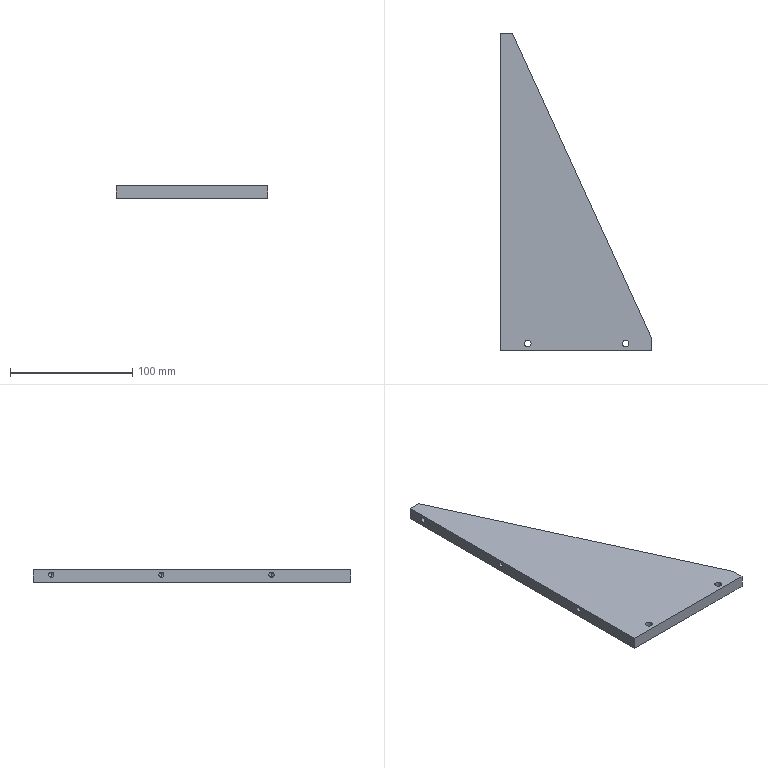Part | STEP file | FBDS-JIN | 1 solid | 29 faces | box 124 x 260 x 10 mm | volume 178303 mm3 | cylinder 14 | plane 9 | cone 6 | commonest cylinder face diameters 4.2 x6 5.5 x4 9.8 x4
STEP:
#1=CARTESIAN_POINT('',(107.4,6.,5.7));
#2=VERTEX_POINT('',#1);
#3=CARTESIAN_POINT('',(97.6,6.,5.7));
#4=VERTEX_POINT('',#3);
#5=CARTESIAN_POINT('',(102.5,6.,5.7));
#6=DIRECTION('',(0.,0.,-1.));
#7=DIRECTION('',(-1.,0.,0.));
#8=AXIS2_PLACEMENT_3D('',#5,#6,#7);
#9=CIRCLE('',#8,4.9);
#10=EDGE_CURVE('',#2,#4,#9,.T.);
#11=ORIENTED_EDGE('',*,*,#10,.F.);
#12=CARTESIAN_POINT('',(107.4,6.,0.));
#13=VERTEX_POINT('',#12);
#14=CARTESIAN_POINT('',(107.4,6.,0.));
#15=DIRECTION('',(0.,0.,-1.));
#16=VECTOR('',#15,1000.);
#17=LINE('',#14,#16);
#18=EDGE_CURVE('',#2,#13,#17,.T.);
#19=ORIENTED_EDGE('',*,*,#18,.T.);
#20=CARTESIAN_POINT('',(97.6,6.,0.));
#21=VERTEX_POINT('',#20);
#22=CARTESIAN_POINT('',(102.5,6.,0.));
#23=DIRECTION('',(0.,0.,-1.));
#24=DIRECTION('',(-1.,0.,0.));
#25=AXIS2_PLACEMENT_3D('',#22,#23,#24);
#26=CIRCLE('',#25,4.9);
#27=EDGE_CURVE('',#13,#21,#26,.T.);
#28=ORIENTED_EDGE('',*,*,#27,.T.);
#29=CARTESIAN_POINT('',(97.6,6.,0.));
#30=DIRECTION('',(0.,0.,-1.));
#31=VECTOR('',#30,1000.);
#32=LINE('',#29,#31);
#33=EDGE_CURVE('',#4,#21,#32,.T.);
#34=ORIENTED_EDGE('',*,*,#33,.F.);
#35=EDGE_LOOP('',(#11,#19,#28,#34));
#36=FACE_OUTER_BOUND('',#35,.T.);
#37=CARTESIAN_POINT('',(102.5,6.,0.));
#38=DIRECTION('',(0.,0.,-1.));
#39=DIRECTION('',(-1.,0.,0.));
#40=AXIS2_PLACEMENT_3D('',#37,#38,#39);
#41=CYLINDRICAL_SURFACE('',#40,4.9);
#42=ADVANCED_FACE('',(#36),#41,.F.);
#43=CARTESIAN_POINT('',(105.25,6.,10.));
#44=VERTEX_POINT('',#43);
#45=CARTESIAN_POINT('',(99.75,6.,10.));
#46=VERTEX_POINT('',#45);
#47=CARTESIAN_POINT('',(102.5,6.,10.));
#48=DIRECTION('',(0.,0.,-1.));
#49=DIRECTION('',(-1.,0.,0.));
#50=AXIS2_PLACEMENT_3D('',#47,#48,#49);
#51=CIRCLE('',#50,2.75);
#52=EDGE_CURVE('',#44,#46,#51,.T.);
#53=ORIENTED_EDGE('',*,*,#52,.F.);
#54=CARTESIAN_POINT('',(105.25,6.,5.7));
#55=VERTEX_POINT('',#54);
#56=CARTESIAN_POINT('',(105.25,6.,0.));
#57=DIRECTION('',(0.,0.,-1.));
#58=VECTOR('',#57,1000.);
#59=LINE('',#56,#58);
#60=EDGE_CURVE('',#44,#55,#59,.T.);
#61=ORIENTED_EDGE('',*,*,#60,.T.);
#62=CARTESIAN_POINT('',(99.75,6.,5.7));
#63=VERTEX_POINT('',#62);
#64=CARTESIAN_POINT('',(102.5,6.,5.7));
#65=DIRECTION('',(0.,0.,-1.));
#66=DIRECTION('',(-1.,0.,0.));
#67=AXIS2_PLACEMENT_3D('',#64,#65,#66);
#68=CIRCLE('',#67,2.75);
#69=EDGE_CURVE('',#55,#63,#68,.T.);
#70=ORIENTED_EDGE('',*,*,#69,.T.);
#71=CARTESIAN_POINT('',(99.75,6.,0.));
#72=DIRECTION('',(0.,0.,-1.));
#73=VECTOR('',#72,1000.);
#74=LINE('',#71,#73);
#75=EDGE_CURVE('',#46,#63,#74,.T.);
#76=ORIENTED_EDGE('',*,*,#75,.F.);
#77=EDGE_LOOP('',(#53,#61,#70,#76));
#78=FACE_OUTER_BOUND('',#77,.T.);
#79=CARTESIAN_POINT('',(102.5,6.,0.));
#80=DIRECTION('',(0.,0.,-1.));
#81=DIRECTION('',(-1.,0.,0.));
#82=AXIS2_PLACEMENT_3D('',#79,#80,#81);
#83=CYLINDRICAL_SURFACE('',#82,2.75);
#84=ADVANCED_FACE('',(#78),#83,.F.);
#85=CARTESIAN_POINT('',(27.4,6.,5.7));
#86=VERTEX_POINT('',#85);
#87=CARTESIAN_POINT('',(17.6,6.,5.7));
#88=VERTEX_POINT('',#87);
#89=CARTESIAN_POINT('',(22.5,6.,5.7));
#90=DIRECTION('',(0.,0.,-1.));
#91=DIRECTION('',(-1.,0.,0.));
#92=AXIS2_PLACEMENT_3D('',#89,#90,#91);
#93=CIRCLE('',#92,4.9);
#94=EDGE_CURVE('',#86,#88,#93,.T.);
#95=ORIENTED_EDGE('',*,*,#94,.F.);
#96=CARTESIAN_POINT('',(27.4,6.,0.));
#97=VERTEX_POINT('',#96);
#98=CARTESIAN_POINT('',(27.4,6.,0.));
#99=DIRECTION('',(0.,0.,-1.));
#100=VECTOR('',#99,1000.);
#101=LINE('',#98,#100);
#102=EDGE_CURVE('',#86,#97,#101,.T.);
#103=ORIENTED_EDGE('',*,*,#102,.T.);
#104=CARTESIAN_POINT('',(17.6,6.,0.));
#105=VERTEX_POINT('',#104);
#106=CARTESIAN_POINT('',(22.5,6.,0.));
#107=DIRECTION('',(0.,0.,-1.));
#108=DIRECTION('',(-1.,0.,0.));
#109=AXIS2_PLACEMENT_3D('',#106,#107,#108);
#110=CIRCLE('',#109,4.9);
#111=EDGE_CURVE('',#97,#105,#110,.T.);
#112=ORIENTED_EDGE('',*,*,#111,.T.);
#113=CARTESIAN_POINT('',(17.6,6.,0.));
#114=DIRECTION('',(0.,0.,-1.));
#115=VECTOR('',#114,1000.);
#116=LINE('',#113,#115);
#117=EDGE_CURVE('',#88,#105,#116,.T.);
#118=ORIENTED_EDGE('',*,*,#117,.F.);
#119=EDGE_LOOP('',(#95,#103,#112,#118));
#120=FACE_OUTER_BOUND('',#119,.T.);
#121=CARTESIAN_POINT('',(22.5,6.,0.));
#122=DIRECTION('',(0.,0.,-1.));
#123=DIRECTION('',(-1.,0.,0.));
#124=AXIS2_PLACEMENT_3D('',#121,#122,#123);
#125=CYLINDRICAL_SURFACE('',#124,4.9);
#126=ADVANCED_FACE('',(#120),#125,.F.);
#127=CARTESIAN_POINT('',(25.25,6.,10.));
#128=VERTEX_POINT('',#127);
#129=CARTESIAN_POINT('',(19.75,6.,10.));
#130=VERTEX_POINT('',#129);
#131=CARTESIAN_POINT('',(22.5,6.,10.));
#132=DIRECTION('',(0.,0.,-1.));
#133=DIRECTION('',(-1.,0.,0.));
#134=AXIS2_PLACEMENT_3D('',#131,#132,#133);
#135=CIRCLE('',#134,2.75);
#136=EDGE_CURVE('',#128,#130,#135,.T.);
#137=ORIENTED_EDGE('',*,*,#136,.F.);
#138=CARTESIAN_POINT('',(25.25,6.,5.7));
#139=VERTEX_POINT('',#138);
#140=CARTESIAN_POINT('',(25.25,6.,0.));
#141=DIRECTION('',(0.,0.,-1.));
#142=VECTOR('',#141,1000.);
#143=LINE('',#140,#142);
#144=EDGE_CURVE('',#128,#139,#143,.T.);
#145=ORIENTED_EDGE('',*,*,#144,.T.);
#146=CARTESIAN_POINT('',(19.75,6.,5.7));
#147=VERTEX_POINT('',#146);
#148=CARTESIAN_POINT('',(22.5,6.,5.7));
#149=DIRECTION('',(0.,0.,-1.));
#150=DIRECTION('',(-1.,0.,0.));
#151=AXIS2_PLACEMENT_3D('',#148,#149,#150);
#152=CIRCLE('',#151,2.75);
#153=EDGE_CURVE('',#139,#147,#152,.T.);
#154=ORIENTED_EDGE('',*,*,#153,.T.);
#155=CARTESIAN_POINT('',(19.75,6.,0.));
#156=DIRECTION('',(0.,0.,-1.));
#157=VECTOR('',#156,1000.);
#158=LINE('',#155,#157);
#159=EDGE_CURVE('',#130,#147,#158,.T.);
#160=ORIENTED_EDGE('',*,*,#159,.F.);
#161=EDGE_LOOP('',(#137,#145,#154,#160));
#162=FACE_OUTER_BOUND('',#161,.T.);
#163=CARTESIAN_POINT('',(22.5,6.,0.));
#164=DIRECTION('',(0.,0.,-1.));
#165=DIRECTION('',(-1.,0.,0.));
#166=AXIS2_PLACEMENT_3D('',#163,#164,#165);
#167=CYLINDRICAL_SURFACE('',#166,2.75);
#168=ADVANCED_FACE('',(#162),#167,.F.);
#169=CARTESIAN_POINT('',(12.4,245.,3.9));
#170=VERTEX_POINT('',#169);
#171=CARTESIAN_POINT('',(12.4,245.,8.1));
#172=VERTEX_POINT('',#171);
#173=CARTESIAN_POINT('',(12.4,245.,6.));
#174=DIRECTION('',(-1.,0.,0.));
#175=DIRECTION('',(0.,0.,1.));
#176=AXIS2_PLACEMENT_3D('',#173,#174,#175);
#177=CIRCLE('',#176,2.1);
#178=EDGE_CURVE('',#170,#172,#177,.T.);
#179=ORIENTED_EDGE('',*,*,#178,.F.);
#180=CARTESIAN_POINT('',(0.,245.,3.9));
#181=VERTEX_POINT('',#180);
#182=CARTESIAN_POINT('',(0.,245.,3.9));
#183=DIRECTION('',(-1.,0.,0.));
#184=VECTOR('',#183,1000.);
#185=LINE('',#182,#184);
#186=EDGE_CURVE('',#170,#181,#185,.T.);
#187=ORIENTED_EDGE('',*,*,#186,.T.);
#188=CARTESIAN_POINT('',(0.,245.,8.1));
#189=VERTEX_POINT('',#188);
#190=CARTESIAN_POINT('',(0.,245.,6.));
#191=DIRECTION('',(-1.,0.,0.));
#192=DIRECTION('',(0.,0.,1.));
#193=AXIS2_PLACEMENT_3D('',#190,#191,#192);
#194=CIRCLE('',#193,2.1);
#195=EDGE_CURVE('',#181,#189,#194,.T.);
#196=ORIENTED_EDGE('',*,*,#195,.T.);
#197=CARTESIAN_POINT('',(0.,245.,8.1));
#198=DIRECTION('',(-1.,0.,0.));
#199=VECTOR('',#198,1000.);
#200=LINE('',#197,#199);
#201=EDGE_CURVE('',#172,#189,#200,.T.);
#202=ORIENTED_EDGE('',*,*,#201,.F.);
#203=EDGE_LOOP('',(#179,#187,#196,#202));
#204=FACE_OUTER_BOUND('',#203,.T.);
#205=CARTESIAN_POINT('',(0.,245.,6.));
#206=DIRECTION('',(-1.,0.,0.));
#207=DIRECTION('',(0.,0.,1.));
#208=AXIS2_PLACEMENT_3D('',#205,#206,#207);
#209=CYLINDRICAL_SURFACE('',#208,2.1);
#210=ADVANCED_FACE('',(#204),#209,.F.);
#211=CARTESIAN_POINT('',(13.662,245.,6.));
#212=VERTEX_POINT('',#211);
#213=CARTESIAN_POINT('',(12.4,245.,8.1));
#214=DIRECTION('',(-0.515,0.,0.8572));
#215=VECTOR('',#214,1000.);
#216=LINE('',#213,#215);
#217=EDGE_CURVE('',#212,#172,#216,.T.);
#218=ORIENTED_EDGE('',*,*,#217,.F.);
#219=CARTESIAN_POINT('',(12.4,245.,3.9));
#220=DIRECTION('',(-0.515,0.,-0.8572));
#221=VECTOR('',#220,1000.);
#222=LINE('',#219,#221);
#223=EDGE_CURVE('',#212,#170,#222,.T.);
#224=ORIENTED_EDGE('',*,*,#223,.T.);
#225=ORIENTED_EDGE('',*,*,#178,.T.);
#226=EDGE_LOOP('',(#218,#224,#225));
#227=FACE_OUTER_BOUND('',#226,.T.);
#228=CARTESIAN_POINT('',(12.4,245.,6.));
#229=DIRECTION('',(-1.,0.,0.));
#230=DIRECTION('',(0.,0.,1.));
#231=AXIS2_PLACEMENT_3D('',#228,#229,#230);
#232=CONICAL_SURFACE('',#231,2.1,1.03);
#233=ADVANCED_FACE('',(#227),#232,.F.);
#234=CARTESIAN_POINT('',(12.4,155.,3.9));
#235=VERTEX_POINT('',#234);
#236=CARTESIAN_POINT('',(12.4,155.,8.1));
#237=VERTEX_POINT('',#236);
#238=CARTESIAN_POINT('',(12.4,155.,6.));
#239=DIRECTION('',(-1.,0.,0.));
#240=DIRECTION('',(0.,0.,1.));
#241=AXIS2_PLACEMENT_3D('',#238,#239,#240);
#242=CIRCLE('',#241,2.1);
#243=EDGE_CURVE('',#235,#237,#242,.T.);
#244=ORIENTED_EDGE('',*,*,#243,.F.);
#245=CARTESIAN_POINT('',(0.,155.,3.9));
#246=VERTEX_POINT('',#245);
#247=CARTESIAN_POINT('',(0.,155.,3.9));
#248=DIRECTION('',(-1.,0.,0.));
#249=VECTOR('',#248,1000.);
#250=LINE('',#247,#249);
#251=EDGE_CURVE('',#235,#246,#250,.T.);
#252=ORIENTED_EDGE('',*,*,#251,.T.);
#253=CARTESIAN_POINT('',(0.,155.,8.1));
#254=VERTEX_POINT('',#253);
#255=CARTESIAN_POINT('',(0.,155.,6.));
#256=DIRECTION('',(-1.,0.,0.));
#257=DIRECTION('',(0.,0.,1.));
#258=AXIS2_PLACEMENT_3D('',#255,#256,#257);
#259=CIRCLE('',#258,2.1);
#260=EDGE_CURVE('',#246,#254,#259,.T.);
#261=ORIENTED_EDGE('',*,*,#260,.T.);
#262=CARTESIAN_POINT('',(0.,155.,8.1));
#263=DIRECTION('',(-1.,0.,0.));
#264=VECTOR('',#263,1000.);
#265=LINE('',#262,#264);
#266=EDGE_CURVE('',#237,#254,#265,.T.);
#267=ORIENTED_EDGE('',*,*,#266,.F.);
#268=EDGE_LOOP('',(#244,#252,#261,#267));
#269=FACE_OUTER_BOUND('',#268,.T.);
#270=CARTESIAN_POINT('',(0.,155.,6.));
#271=DIRECTION('',(-1.,0.,0.));
#272=DIRECTION('',(0.,0.,1.));
#273=AXIS2_PLACEMENT_3D('',#270,#271,#272);
#274=CYLINDRICAL_SURFACE('',#273,2.1);
#275=ADVANCED_FACE('',(#269),#274,.F.);
#276=CARTESIAN_POINT('',(13.662,155.,6.));
#277=VERTEX_POINT('',#276);
#278=CARTESIAN_POINT('',(12.4,155.,8.1));
#279=DIRECTION('',(-0.515,0.,0.8572));
#280=VECTOR('',#279,1000.);
#281=LINE('',#278,#280);
#282=EDGE_CURVE('',#277,#237,#281,.T.);
#283=ORIENTED_EDGE('',*,*,#282,.F.);
#284=CARTESIAN_POINT('',(12.4,155.,3.9));
#285=DIRECTION('',(-0.515,0.,-0.8572));
#286=VECTOR('',#285,1000.);
#287=LINE('',#284,#286);
#288=EDGE_CURVE('',#277,#235,#287,.T.);
#289=ORIENTED_EDGE('',*,*,#288,.T.);
#290=ORIENTED_EDGE('',*,*,#243,.T.);
#291=EDGE_LOOP('',(#283,#289,#290));
#292=FACE_OUTER_BOUND('',#291,.T.);
#293=CARTESIAN_POINT('',(12.4,155.,6.));
#294=DIRECTION('',(-1.,0.,0.));
#295=DIRECTION('',(0.,0.,1.));
#296=AXIS2_PLACEMENT_3D('',#293,#294,#295);
#297=CONICAL_SURFACE('',#296,2.1,1.03);
#298=ADVANCED_FACE('',(#292),#297,.F.);
#299=CARTESIAN_POINT('',(12.4,65.,3.9));
#300=VERTEX_POINT('',#299);
#301=CARTESIAN_POINT('',(12.4,65.,8.1));
#302=VERTEX_POINT('',#301);
#303=CARTESIAN_POINT('',(12.4,65.,6.));
#304=DIRECTION('',(-1.,0.,0.));
#305=DIRECTION('',(0.,0.,1.));
#306=AXIS2_PLACEMENT_3D('',#303,#304,#305);
#307=CIRCLE('',#306,2.1);
#308=EDGE_CURVE('',#300,#302,#307,.T.);
#309=ORIENTED_EDGE('',*,*,#308,.F.);
#310=CARTESIAN_POINT('',(0.,65.,3.9));
#311=VERTEX_POINT('',#310);
#312=CARTESIAN_POINT('',(0.,65.,3.9));
#313=DIRECTION('',(-1.,0.,0.));
#314=VECTOR('',#313,1000.);
#315=LINE('',#312,#314);
#316=EDGE_CURVE('',#300,#311,#315,.T.);
#317=ORIENTED_EDGE('',*,*,#316,.T.);
#318=CARTESIAN_POINT('',(0.,65.,8.1));
#319=VERTEX_POINT('',#318);
#320=CARTESIAN_POINT('',(0.,65.,6.));
#321=DIRECTION('',(-1.,0.,0.));
#322=DIRECTION('',(0.,0.,1.));
#323=AXIS2_PLACEMENT_3D('',#320,#321,#322);
#324=CIRCLE('',#323,2.1);
#325=EDGE_CURVE('',#311,#319,#324,.T.);
#326=ORIENTED_EDGE('',*,*,#325,.T.);
#327=CARTESIAN_POINT('',(0.,65.,8.1));
#328=DIRECTION('',(-1.,0.,0.));
#329=VECTOR('',#328,1000.);
#330=LINE('',#327,#329);
#331=EDGE_CURVE('',#302,#319,#330,.T.);
#332=ORIENTED_EDGE('',*,*,#331,.F.);
#333=EDGE_LOOP('',(#309,#317,#326,#332));
#334=FACE_OUTER_BOUND('',#333,.T.);
#335=CARTESIAN_POINT('',(0.,65.,6.));
#336=DIRECTION('',(-1.,0.,0.));
#337=DIRECTION('',(0.,0.,1.));
#338=AXIS2_PLACEMENT_3D('',#335,#336,#337);
#339=CYLINDRICAL_SURFACE('',#338,2.1);
#340=ADVANCED_FACE('',(#334),#339,.F.);
#341=CARTESIAN_POINT('',(13.662,65.,6.));
#342=VERTEX_POINT('',#341);
#343=CARTESIAN_POINT('',(12.4,65.,8.1));
#344=DIRECTION('',(-0.515,0.,0.8572));
#345=VECTOR('',#344,1000.);
#346=LINE('',#343,#345);
#347=EDGE_CURVE('',#342,#302,#346,.T.);
#348=ORIENTED_EDGE('',*,*,#347,.F.);
#349=CARTESIAN_POINT('',(12.4,65.,3.9));
#350=DIRECTION('',(-0.515,0.,-0.8572));
#351=VECTOR('',#350,1000.);
#352=LINE('',#349,#351);
#353=EDGE_CURVE('',#342,#300,#352,.T.);
#354=ORIENTED_EDGE('',*,*,#353,.T.);
#355=ORIENTED_EDGE('',*,*,#308,.T.);
#356=EDGE_LOOP('',(#348,#354,#355));
#357=FACE_OUTER_BOUND('',#356,.T.);
#358=CARTESIAN_POINT('',(12.4,65.,6.));
#359=DIRECTION('',(-1.,0.,0.));
#360=DIRECTION('',(0.,0.,1.));
#361=AXIS2_PLACEMENT_3D('',#358,#359,#360);
#362=CONICAL_SURFACE('',#361,2.1,1.03);
#363=ADVANCED_FACE('',(#357),#362,.F.);
#364=CARTESIAN_POINT('',(0.,245.,6.));
#365=DIRECTION('',(-1.,0.,0.));
#366=DIRECTION('',(0.,0.,1.));
#367=AXIS2_PLACEMENT_3D('',#364,#365,#366);
#368=CIRCLE('',#367,2.1);
#369=EDGE_CURVE('',#189,#181,#368,.T.);
#370=ORIENTED_EDGE('',*,*,#369,.F.);
#371=ORIENTED_EDGE('',*,*,#195,.F.);
#372=EDGE_LOOP('',(#370,#371));
#373=FACE_BOUND('',#372,.T.);
#374=CARTESIAN_POINT('',(0.,155.,6.));
#375=DIRECTION('',(-1.,0.,0.));
#376=DIRECTION('',(0.,0.,1.));
#377=AXIS2_PLACEMENT_3D('',#374,#375,#376);
#378=CIRCLE('',#377,2.1);
#379=EDGE_CURVE('',#254,#246,#378,.T.);
#380=ORIENTED_EDGE('',*,*,#379,.F.);
#381=ORIENTED_EDGE('',*,*,#260,.F.);
#382=EDGE_LOOP('',(#380,#381));
#383=FACE_BOUND('',#382,.T.);
#384=CARTESIAN_POINT('',(0.,65.,6.));
#385=DIRECTION('',(-1.,0.,0.));
#386=DIRECTION('',(0.,0.,1.));
#387=AXIS2_PLACEMENT_3D('',#384,#385,#386);
#388=CIRCLE('',#387,2.1);
#389=EDGE_CURVE('',#319,#311,#388,.T.);
#390=ORIENTED_EDGE('',*,*,#389,.F.);
#391=ORIENTED_EDGE('',*,*,#325,.F.);
#392=EDGE_LOOP('',(#390,#391));
#393=FACE_BOUND('',#392,.T.);
#394=CARTESIAN_POINT('',(0.,260.,0.));
#395=VERTEX_POINT('',#394);
#396=CARTESIAN_POINT('',(0.,0.,0.));
#397=VERTEX_POINT('',#396);
#398=CARTESIAN_POINT('',(0.,0.,0.));
#399=DIRECTION('',(0.,-1.,0.));
#400=VECTOR('',#399,1000.);
#401=LINE('',#398,#400);
#402=EDGE_CURVE('',#395,#397,#401,.T.);
#403=ORIENTED_EDGE('',*,*,#402,.T.);
#404=CARTESIAN_POINT('',(0.,0.,10.));
#405=VERTEX_POINT('',#404);
#406=CARTESIAN_POINT('',(0.,0.,10.));
#407=DIRECTION('',(0.,0.,-1.));
#408=VECTOR('',#407,1000.);
#409=LINE('',#406,#408);
#410=EDGE_CURVE('',#405,#397,#409,.T.);
#411=ORIENTED_EDGE('',*,*,#410,.F.);
#412=CARTESIAN_POINT('',(0.,260.,10.));
#413=VERTEX_POINT('',#412);
#414=CARTESIAN_POINT('',(0.,0.,10.));
#415=DIRECTION('',(0.,-1.,0.));
#416=VECTOR('',#415,1000.);
#417=LINE('',#414,#416);
#418=EDGE_CURVE('',#413,#405,#417,.T.);
#419=ORIENTED_EDGE('',*,*,#418,.F.);
#420=CARTESIAN_POINT('',(0.,260.,10.));
#421=DIRECTION('',(0.,0.,-1.));
#422=VECTOR('',#421,1000.);
#423=LINE('',#420,#422);
#424=EDGE_CURVE('',#413,#395,#423,.T.);
#425=ORIENTED_EDGE('',*,*,#424,.T.);
#426=EDGE_LOOP('',(#403,#411,#419,#425));
#427=FACE_OUTER_BOUND('',#426,.T.);
#428=CARTESIAN_POINT('',(0.,0.,10.));
#429=DIRECTION('',(1.,0.,0.));
#430=DIRECTION('',(0.,0.,-1.));
#431=AXIS2_PLACEMENT_3D('',#428,#429,#430);
#432=PLANE('',#431);
#433=ADVANCED_FACE('',(#373,#383,#393,#427),#432,.F.);
#434=CARTESIAN_POINT('',(124.,0.,0.));
#435=VERTEX_POINT('',#434);
#436=CARTESIAN_POINT('',(0.,0.,0.));
#437=DIRECTION('',(1.,0.,0.));
#438=VECTOR('',#437,1000.);
#439=LINE('',#436,#438);
#440=EDGE_CURVE('',#397,#435,#439,.T.);
#441=ORIENTED_EDGE('',*,*,#440,.T.);
#442=CARTESIAN_POINT('',(124.,0.,10.));
#443=VERTEX_POINT('',#442);
#444=CARTESIAN_POINT('',(124.,0.,10.));
#445=DIRECTION('',(0.,0.,-1.));
#446=VECTOR('',#445,1000.);
#447=LINE('',#444,#446);
#448=EDGE_CURVE('',#443,#435,#447,.T.);
#449=ORIENTED_EDGE('',*,*,#448,.F.);
#450=CARTESIAN_POINT('',(0.,0.,10.));
#451=DIRECTION('',(1.,0.,0.));
#452=VECTOR('',#451,1000.);
#453=LINE('',#450,#452);
#454=EDGE_CURVE('',#405,#443,#453,.T.);
#455=ORIENTED_EDGE('',*,*,#454,.F.);
#456=ORIENTED_EDGE('',*,*,#410,.T.);
#457=EDGE_LOOP('',(#441,#449,#455,#456));
#458=FACE_OUTER_BOUND('',#457,.T.);
#459=CARTESIAN_POINT('',(0.,0.,10.));
#460=DIRECTION('',(0.,1.,0.));
#461=DIRECTION('',(0.,0.,1.));
#462=AXIS2_PLACEMENT_3D('',#459,#460,#461);
#463=PLANE('',#462);
#464=ADVANCED_FACE('',(#458),#463,.F.);
#465=CARTESIAN_POINT('',(124.,10.,0.));
#466=VERTEX_POINT('',#465);
#467=CARTESIAN_POINT('',(124.,0.,0.));
#468=DIRECTION('',(0.,1.,0.));
#469=VECTOR('',#468,1000.);
#470=LINE('',#467,#469);
#471=EDGE_CURVE('',#435,#466,#470,.T.);
#472=ORIENTED_EDGE('',*,*,#471,.T.);
#473=CARTESIAN_POINT('',(124.,10.,10.));
#474=VERTEX_POINT('',#473);
#475=CARTESIAN_POINT('',(124.,10.,10.));
#476=DIRECTION('',(0.,0.,-1.));
#477=VECTOR('',#476,1000.);
#478=LINE('',#475,#477);
#479=EDGE_CURVE('',#474,#466,#478,.T.);
#480=ORIENTED_EDGE('',*,*,#479,.F.);
#481=CARTESIAN_POINT('',(124.,0.,10.));
#482=DIRECTION('',(0.,1.,0.));
#483=VECTOR('',#482,1000.);
#484=LINE('',#481,#483);
#485=EDGE_CURVE('',#443,#474,#484,.T.);
#486=ORIENTED_EDGE('',*,*,#485,.F.);
#487=ORIENTED_EDGE('',*,*,#448,.T.);
#488=EDGE_LOOP('',(#472,#480,#486,#487));
#489=FACE_OUTER_BOUND('',#488,.T.);
#490=CARTESIAN_POINT('',(124.,0.,10.));
#491=DIRECTION('',(-1.,0.,0.));
#492=DIRECTION('',(0.,0.,1.));
#493=AXIS2_PLACEMENT_3D('',#490,#491,#492);
#494=PLANE('',#493);
#495=ADVANCED_FACE('',(#489),#494,.F.);
#496=CARTESIAN_POINT('',(10.,260.,0.));
#497=VERTEX_POINT('',#496);
#498=CARTESIAN_POINT('',(124.,10.,0.));
#499=DIRECTION('',(-0.4149,0.9099,0.));
#500=VECTOR('',#499,1000.);
#501=LINE('',#498,#500);
#502=EDGE_CURVE('',#466,#497,#501,.T.);
#503=ORIENTED_EDGE('',*,*,#502,.T.);
#504=CARTESIAN_POINT('',(10.,260.,10.));
#505=VERTEX_POINT('',#504);
#506=CARTESIAN_POINT('',(10.,260.,10.));
#507=DIRECTION('',(0.,0.,-1.));
#508=VECTOR('',#507,1000.);
#509=LINE('',#506,#508);
#510=EDGE_CURVE('',#505,#497,#509,.T.);
#511=ORIENTED_EDGE('',*,*,#510,.F.);
#512=CARTESIAN_POINT('',(124.,10.,10.));
#513=DIRECTION('',(-0.4149,0.9099,0.));
#514=VECTOR('',#513,1000.);
#515=LINE('',#512,#514);
#516=EDGE_CURVE('',#474,#505,#515,.T.);
#517=ORIENTED_EDGE('',*,*,#516,.F.);
#518=ORIENTED_EDGE('',*,*,#479,.T.);
#519=EDGE_LOOP('',(#503,#511,#517,#518));
#520=FACE_OUTER_BOUND('',#519,.T.);
#521=CARTESIAN_POINT('',(124.,10.,10.));
#522=DIRECTION('',(-0.9099,-0.4149,0.));
#523=DIRECTION('',(0.4149,-0.9099,0.));
#524=AXIS2_PLACEMENT_3D('',#521,#522,#523);
#525=PLANE('',#524);
#526=ADVANCED_FACE('',(#520),#525,.F.);
#527=CARTESIAN_POINT('',(0.,260.,0.));
#528=DIRECTION('',(-1.,0.,0.));
#529=VECTOR('',#528,1000.);
#530=LINE('',#527,#529);
#531=EDGE_CURVE('',#497,#395,#530,.T.);
#532=ORIENTED_EDGE('',*,*,#531,.T.);
#533=ORIENTED_EDGE('',*,*,#424,.F.);
#534=CARTESIAN_POINT('',(0.,260.,10.));
#535=DIRECTION('',(-1.,0.,0.));
#536=VECTOR('',#535,1000.);
#537=LINE('',#534,#536);
#538=EDGE_CURVE('',#505,#413,#537,.T.);
#539=ORIENTED_EDGE('',*,*,#538,.F.);
#540=ORIENTED_EDGE('',*,*,#510,.T.);
#541=EDGE_LOOP('',(#532,#533,#539,#540));
#542=FACE_OUTER_BOUND('',#541,.T.);
#543=CARTESIAN_POINT('',(0.,260.,10.));
#544=DIRECTION('',(0.,-1.,0.));
#545=DIRECTION('',(0.,0.,-1.));
#546=AXIS2_PLACEMENT_3D('',#543,#544,#545);
#547=PLANE('',#546);
#548=ADVANCED_FACE('',(#542),#547,.F.);
#549=CARTESIAN_POINT('',(102.5,6.,10.));
#550=DIRECTION('',(0.,0.,-1.));
#551=DIRECTION('',(-1.,0.,0.));
#552=AXIS2_PLACEMENT_3D('',#549,#550,#551);
#553=CIRCLE('',#552,2.75);
#554=EDGE_CURVE('',#46,#44,#553,.T.);
#555=ORIENTED_EDGE('',*,*,#554,.T.);
#556=ORIENTED_EDGE('',*,*,#52,.T.);
#557=EDGE_LOOP('',(#555,#556));
#558=FACE_BOUND('',#557,.T.);
#559=CARTESIAN_POINT('',(22.5,6.,10.));
#560=DIRECTION('',(0.,0.,-1.));
#561=DIRECTION('',(-1.,0.,0.));
#562=AXIS2_PLACEMENT_3D('',#559,#560,#561);
#563=CIRCLE('',#562,2.75);
#564=EDGE_CURVE('',#130,#128,#563,.T.);
#565=ORIENTED_EDGE('',*,*,#564,.T.);
#566=ORIENTED_EDGE('',*,*,#136,.T.);
#567=EDGE_LOOP('',(#565,#566));
#568=FACE_BOUND('',#567,.T.);
#569=ORIENTED_EDGE('',*,*,#418,.T.);
#570=ORIENTED_EDGE('',*,*,#454,.T.);
#571=ORIENTED_EDGE('',*,*,#485,.T.);
#572=ORIENTED_EDGE('',*,*,#516,.T.);
#573=ORIENTED_EDGE('',*,*,#538,.T.);
#574=EDGE_LOOP('',(#569,#570,#571,#572,#573));
#575=FACE_OUTER_BOUND('',#574,.T.);
#576=CARTESIAN_POINT('',(0.,0.,10.));
#577=DIRECTION('',(0.,0.,-1.));
#578=DIRECTION('',(-1.,0.,0.));
#579=AXIS2_PLACEMENT_3D('',#576,#577,#578);
#580=PLANE('',#579);
#581=ADVANCED_FACE('',(#558,#568,#575),#580,.F.);
#582=CARTESIAN_POINT('',(102.5,6.,0.));
#583=DIRECTION('',(0.,0.,-1.));
#584=DIRECTION('',(-1.,0.,0.));
#585=AXIS2_PLACEMENT_3D('',#582,#583,#584);
#586=CIRCLE('',#585,4.9);
#587=EDGE_CURVE('',#21,#13,#586,.T.);
#588=ORIENTED_EDGE('',*,*,#587,.F.);
#589=ORIENTED_EDGE('',*,*,#27,.F.);
#590=EDGE_LOOP('',(#588,#589));
#591=FACE_BOUND('',#590,.T.);
#592=CARTESIAN_POINT('',(22.5,6.,0.));
#593=DIRECTION('',(0.,0.,-1.));
#594=DIRECTION('',(-1.,0.,0.));
#595=AXIS2_PLACEMENT_3D('',#592,#593,#594);
#596=CIRCLE('',#595,4.9);
#597=EDGE_CURVE('',#105,#97,#596,.T.);
#598=ORIENTED_EDGE('',*,*,#597,.F.);
#599=ORIENTED_EDGE('',*,*,#111,.F.);
#600=EDGE_LOOP('',(#598,#599));
#601=FACE_BOUND('',#600,.T.);
#602=ORIENTED_EDGE('',*,*,#402,.F.);
#603=ORIENTED_EDGE('',*,*,#531,.F.);
#604=ORIENTED_EDGE('',*,*,#502,.F.);
#605=ORIENTED_EDGE('',*,*,#471,.F.);
#606=ORIENTED_EDGE('',*,*,#440,.F.);
#607=EDGE_LOOP('',(#602,#603,#604,#605,#606));
#608=FACE_OUTER_BOUND('',#607,.T.);
#609=CARTESIAN_POINT('',(0.,0.,0.));
#610=DIRECTION('',(0.,0.,-1.));
#611=DIRECTION('',(-1.,0.,0.));
#612=AXIS2_PLACEMENT_3D('',#609,#610,#611);
#613=PLANE('',#612);
#614=ADVANCED_FACE('',(#591,#601,#608),#613,.T.);
#615=ORIENTED_EDGE('',*,*,#353,.F.);
#616=ORIENTED_EDGE('',*,*,#347,.T.);
#617=CARTESIAN_POINT('',(12.4,65.,6.));
#618=DIRECTION('',(-1.,0.,0.));
#619=DIRECTION('',(0.,0.,1.));
#620=AXIS2_PLACEMENT_3D('',#617,#618,#619);
#621=CIRCLE('',#620,2.1);
#622=EDGE_CURVE('',#302,#300,#621,.T.);
#623=ORIENTED_EDGE('',*,*,#622,.T.);
#624=EDGE_LOOP('',(#615,#616,#623));
#625=FACE_OUTER_BOUND('',#624,.T.);
#626=CARTESIAN_POINT('',(12.4,65.,6.));
#627=DIRECTION('',(-1.,0.,0.));
#628=DIRECTION('',(0.,0.,1.));
#629=AXIS2_PLACEMENT_3D('',#626,#627,#628);
#630=CONICAL_SURFACE('',#629,2.1,1.03);
#631=ADVANCED_FACE('',(#625),#630,.F.);
#632=ORIENTED_EDGE('',*,*,#316,.F.);
#633=ORIENTED_EDGE('',*,*,#622,.F.);
#634=ORIENTED_EDGE('',*,*,#331,.T.);
#635=ORIENTED_EDGE('',*,*,#389,.T.);
#636=EDGE_LOOP('',(#632,#633,#634,#635));
#637=FACE_OUTER_BOUND('',#636,.T.);
#638=CARTESIAN_POINT('',(0.,65.,6.));
#639=DIRECTION('',(-1.,0.,0.));
#640=DIRECTION('',(0.,0.,1.));
#641=AXIS2_PLACEMENT_3D('',#638,#639,#640);
#642=CYLINDRICAL_SURFACE('',#641,2.1);
#643=ADVANCED_FACE('',(#637),#642,.F.);
#644=ORIENTED_EDGE('',*,*,#288,.F.);
#645=ORIENTED_EDGE('',*,*,#282,.T.);
#646=CARTESIAN_POINT('',(12.4,155.,6.));
#647=DIRECTION('',(-1.,0.,0.));
#648=DIRECTION('',(0.,0.,1.));
#649=AXIS2_PLACEMENT_3D('',#646,#647,#648);
#650=CIRCLE('',#649,2.1);
#651=EDGE_CURVE('',#237,#235,#650,.T.);
#652=ORIENTED_EDGE('',*,*,#651,.T.);
#653=EDGE_LOOP('',(#644,#645,#652));
#654=FACE_OUTER_BOUND('',#653,.T.);
#655=CARTESIAN_POINT('',(12.4,155.,6.));
#656=DIRECTION('',(-1.,0.,0.));
#657=DIRECTION('',(0.,0.,1.));
#658=AXIS2_PLACEMENT_3D('',#655,#656,#657);
#659=CONICAL_SURFACE('',#658,2.1,1.03);
#660=ADVANCED_FACE('',(#654),#659,.F.);
#661=ORIENTED_EDGE('',*,*,#251,.F.);
#662=ORIENTED_EDGE('',*,*,#651,.F.);
#663=ORIENTED_EDGE('',*,*,#266,.T.);
#664=ORIENTED_EDGE('',*,*,#379,.T.);
#665=EDGE_LOOP('',(#661,#662,#663,#664));
#666=FACE_OUTER_BOUND('',#665,.T.);
#667=CARTESIAN_POINT('',(0.,155.,6.));
#668=DIRECTION('',(-1.,0.,0.));
#669=DIRECTION('',(0.,0.,1.));
#670=AXIS2_PLACEMENT_3D('',#667,#668,#669);
#671=CYLINDRICAL_SURFACE('',#670,2.1);
#672=ADVANCED_FACE('',(#666),#671,.F.);
#673=ORIENTED_EDGE('',*,*,#223,.F.);
#674=ORIENTED_EDGE('',*,*,#217,.T.);
#675=CARTESIAN_POINT('',(12.4,245.,6.));
#676=DIRECTION('',(-1.,0.,0.));
#677=DIRECTION('',(0.,0.,1.));
#678=AXIS2_PLACEMENT_3D('',#675,#676,#677);
#679=CIRCLE('',#678,2.1);
#680=EDGE_CURVE('',#172,#170,#679,.T.);
#681=ORIENTED_EDGE('',*,*,#680,.T.);
#682=EDGE_LOOP('',(#673,#674,#681));
#683=FACE_OUTER_BOUND('',#682,.T.);
#684=CARTESIAN_POINT('',(12.4,245.,6.));
#685=DIRECTION('',(-1.,0.,0.));
#686=DIRECTION('',(0.,0.,1.));
#687=AXIS2_PLACEMENT_3D('',#684,#685,#686);
#688=CONICAL_SURFACE('',#687,2.1,1.03);
#689=ADVANCED_FACE('',(#683),#688,.F.);
#690=ORIENTED_EDGE('',*,*,#186,.F.);
#691=ORIENTED_EDGE('',*,*,#680,.F.);
#692=ORIENTED_EDGE('',*,*,#201,.T.);
#693=ORIENTED_EDGE('',*,*,#369,.T.);
#694=EDGE_LOOP('',(#690,#691,#692,#693));
#695=FACE_OUTER_BOUND('',#694,.T.);
#696=CARTESIAN_POINT('',(0.,245.,6.));
#697=DIRECTION('',(-1.,0.,0.));
#698=DIRECTION('',(0.,0.,1.));
#699=AXIS2_PLACEMENT_3D('',#696,#697,#698);
#700=CYLINDRICAL_SURFACE('',#699,2.1);
#701=ADVANCED_FACE('',(#695),#700,.F.);
#702=ORIENTED_EDGE('',*,*,#144,.F.);
#703=ORIENTED_EDGE('',*,*,#564,.F.);
#704=ORIENTED_EDGE('',*,*,#159,.T.);
#705=CARTESIAN_POINT('',(22.5,6.,5.7));
#706=DIRECTION('',(0.,0.,-1.));
#707=DIRECTION('',(-1.,0.,0.));
#708=AXIS2_PLACEMENT_3D('',#705,#706,#707);
#709=CIRCLE('',#708,2.75);
#710=EDGE_CURVE('',#147,#139,#709,.T.);
#711=ORIENTED_EDGE('',*,*,#710,.T.);
#712=EDGE_LOOP('',(#702,#703,#704,#711));
#713=FACE_OUTER_BOUND('',#712,.T.);
#714=CARTESIAN_POINT('',(22.5,6.,0.));
#715=DIRECTION('',(0.,0.,-1.));
#716=DIRECTION('',(-1.,0.,0.));
#717=AXIS2_PLACEMENT_3D('',#714,#715,#716);
#718=CYLINDRICAL_SURFACE('',#717,2.75);
#719=ADVANCED_FACE('',(#713),#718,.F.);
#720=ORIENTED_EDGE('',*,*,#710,.F.);
#721=ORIENTED_EDGE('',*,*,#153,.F.);
#722=EDGE_LOOP('',(#720,#721));
#723=FACE_BOUND('',#722,.T.);
#724=CARTESIAN_POINT('',(22.5,6.,5.7));
#725=DIRECTION('',(0.,0.,-1.));
#726=DIRECTION('',(-1.,0.,0.));
#727=AXIS2_PLACEMENT_3D('',#724,#725,#726);
#728=CIRCLE('',#727,4.9);
#729=EDGE_CURVE('',#88,#86,#728,.T.);
#730=ORIENTED_EDGE('',*,*,#729,.T.);
#731=ORIENTED_EDGE('',*,*,#94,.T.);
#732=EDGE_LOOP('',(#730,#731));
#733=FACE_OUTER_BOUND('',#732,.T.);
#734=CARTESIAN_POINT('',(25.25,6.,5.7));
#735=DIRECTION('',(0.,0.,1.));
#736=DIRECTION('',(1.,0.,0.));
#737=AXIS2_PLACEMENT_3D('',#734,#735,#736);
#738=PLANE('',#737);
#739=ADVANCED_FACE('',(#723,#733),#738,.F.);
#740=ORIENTED_EDGE('',*,*,#102,.F.);
#741=ORIENTED_EDGE('',*,*,#729,.F.);
#742=ORIENTED_EDGE('',*,*,#117,.T.);
#743=ORIENTED_EDGE('',*,*,#597,.T.);
#744=EDGE_LOOP('',(#740,#741,#742,#743));
#745=FACE_OUTER_BOUND('',#744,.T.);
#746=CARTESIAN_POINT('',(22.5,6.,0.));
#747=DIRECTION('',(0.,0.,-1.));
#748=DIRECTION('',(-1.,0.,0.));
#749=AXIS2_PLACEMENT_3D('',#746,#747,#748);
#750=CYLINDRICAL_SURFACE('',#749,4.9);
#751=ADVANCED_FACE('',(#745),#750,.F.);
#752=ORIENTED_EDGE('',*,*,#60,.F.);
#753=ORIENTED_EDGE('',*,*,#554,.F.);
#754=ORIENTED_EDGE('',*,*,#75,.T.);
#755=CARTESIAN_POINT('',(102.5,6.,5.7));
#756=DIRECTION('',(0.,0.,-1.));
#757=DIRECTION('',(-1.,0.,0.));
#758=AXIS2_PLACEMENT_3D('',#755,#756,#757);
#759=CIRCLE('',#758,2.75);
#760=EDGE_CURVE('',#63,#55,#759,.T.);
#761=ORIENTED_EDGE('',*,*,#760,.T.);
#762=EDGE_LOOP('',(#752,#753,#754,#761));
#763=FACE_OUTER_BOUND('',#762,.T.);
#764=CARTESIAN_POINT('',(102.5,6.,0.));
#765=DIRECTION('',(0.,0.,-1.));
#766=DIRECTION('',(-1.,0.,0.));
#767=AXIS2_PLACEMENT_3D('',#764,#765,#766);
#768=CYLINDRICAL_SURFACE('',#767,2.75);
#769=ADVANCED_FACE('',(#763),#768,.F.);
#770=ORIENTED_EDGE('',*,*,#760,.F.);
#771=ORIENTED_EDGE('',*,*,#69,.F.);
#772=EDGE_LOOP('',(#770,#771));
#773=FACE_BOUND('',#772,.T.);
#774=CARTESIAN_POINT('',(102.5,6.,5.7));
#775=DIRECTION('',(0.,0.,-1.));
#776=DIRECTION('',(-1.,0.,0.));
#777=AXIS2_PLACEMENT_3D('',#774,#775,#776);
#778=CIRCLE('',#777,4.9);
#779=EDGE_CURVE('',#4,#2,#778,.T.);
#780=ORIENTED_EDGE('',*,*,#779,.T.);
#781=ORIENTED_EDGE('',*,*,#10,.T.);
#782=EDGE_LOOP('',(#780,#781));
#783=FACE_OUTER_BOUND('',#782,.T.);
#784=CARTESIAN_POINT('',(105.25,6.,5.7));
#785=DIRECTION('',(0.,0.,1.));
#786=DIRECTION('',(1.,0.,0.));
#787=AXIS2_PLACEMENT_3D('',#784,#785,#786);
#788=PLANE('',#787);
#789=ADVANCED_FACE('',(#773,#783),#788,.F.);
#790=ORIENTED_EDGE('',*,*,#18,.F.);
#791=ORIENTED_EDGE('',*,*,#779,.F.);
#792=ORIENTED_EDGE('',*,*,#33,.T.);
#793=ORIENTED_EDGE('',*,*,#587,.T.);
#794=EDGE_LOOP('',(#790,#791,#792,#793));
#795=FACE_OUTER_BOUND('',#794,.T.);
#796=CARTESIAN_POINT('',(102.5,6.,0.));
#797=DIRECTION('',(0.,0.,-1.));
#798=DIRECTION('',(-1.,0.,0.));
#799=AXIS2_PLACEMENT_3D('',#796,#797,#798);
#800=CYLINDRICAL_SURFACE('',#799,4.9);
#801=ADVANCED_FACE('',(#795),#800,.F.);
#802=CLOSED_SHELL('',(#42,#84,#126,#168,#210,#233,#275,#298,#340,#363,#433,#464,#495,#526,#548,#581,#614,#631,#643,#660,#672,#689,#701,#719,#739,#751,#769,#789,#801));
#803=MANIFOLD_SOLID_BREP('',#802);
#804=CARTESIAN_POINT('',(0.,0.,0.));
#805=DIRECTION('',(0.,0.,1.));
#806=DIRECTION('',(1.,0.,0.));
#807=AXIS2_PLACEMENT_3D('',#804,#805,#806);
#808=(LENGTH_UNIT()NAMED_UNIT(*)SI_UNIT(.MILLI.,.METRE.));
#809=UNCERTAINTY_MEASURE_WITH_UNIT(LENGTH_MEASURE(0.00001),#808,'','');
#810=(NAMED_UNIT(*)PLANE_ANGLE_UNIT()SI_UNIT($,.RADIAN.));
#811=(NAMED_UNIT(*)SI_UNIT($,.STERADIAN.)SOLID_ANGLE_UNIT());
#812=(GEOMETRIC_REPRESENTATION_CONTEXT(3)GLOBAL_UNCERTAINTY_ASSIGNED_CONTEXT((#809))GLOBAL_UNIT_ASSIGNED_CONTEXT((#808,#810,#811))REPRESENTATION_CONTEXT('',''));
#813=ADVANCED_BREP_SHAPE_REPRESENTATION('',(#803,#807),#812);